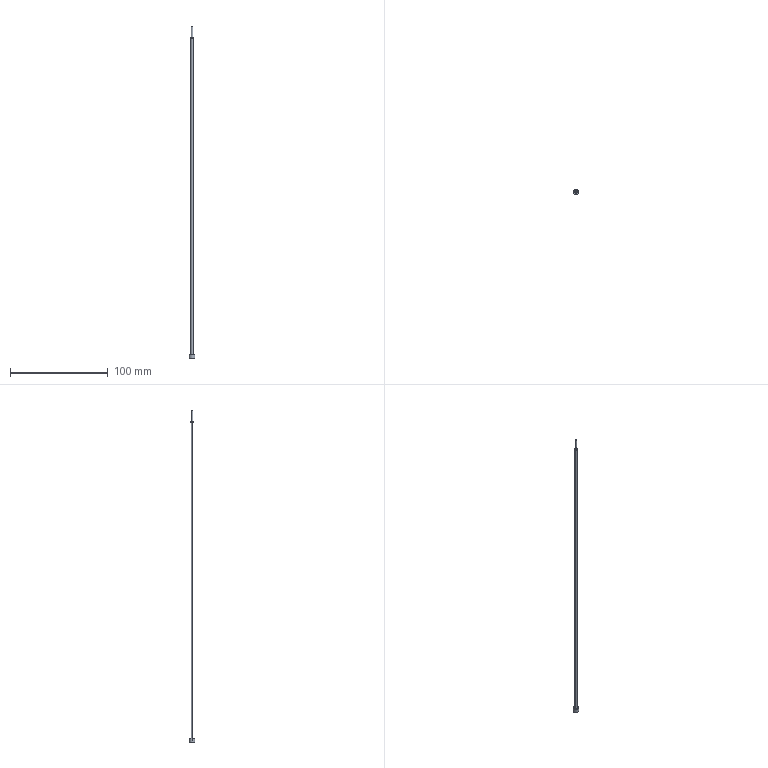Part | Creo | 1 solid | 13 faces | box 6 x 6 x 339.574 mm | volume 2143 mm3 | plane 5 | cone 4 | cylinder 4 | commonest cylinder face diameters 2.8 x2 6 x2
STEP:
#1=CARTESIAN_POINT('',(49.138,56.28,-20.728));
#2=VERTEX_POINT('',#1);
#3=CARTESIAN_POINT('',(46.338,56.28,-20.728));
#4=VERTEX_POINT('',#3);
#5=CARTESIAN_POINT('',(47.738,56.28,-20.728));
#6=DIRECTION('',(0.,0.,1.));
#7=DIRECTION('',(1.,0.,0.));
#8=AXIS2_PLACEMENT_3D('',#5,#6,#7);
#9=CIRCLE('',#8,1.4);
#10=EDGE_CURVE('',#2,#4,#9,.T.);
#11=ORIENTED_EDGE('',*,*,#10,.F.);
#12=CARTESIAN_POINT('',(47.738,56.28,-20.728));
#13=DIRECTION('',(0.,0.,1.));
#14=DIRECTION('',(-1.,0.,0.));
#15=AXIS2_PLACEMENT_3D('',#12,#13,#14);
#16=CIRCLE('',#15,1.4);
#17=EDGE_CURVE('',#4,#2,#16,.T.);
#18=ORIENTED_EDGE('',*,*,#17,.F.);
#19=EDGE_LOOP('',(#11,#18));
#20=FACE_OUTER_BOUND('',#19,.F.);
#21=CARTESIAN_POINT('',(49.1,56.28,-20.728));
#22=VERTEX_POINT('',#21);
#23=CARTESIAN_POINT('',(46.375,56.28,-20.728));
#24=VERTEX_POINT('',#23);
#25=CARTESIAN_POINT('',(47.737,56.28,-20.728));
#26=DIRECTION('',(0.,0.,-1.));
#27=DIRECTION('',(1.,0.,0.));
#28=AXIS2_PLACEMENT_3D('',#25,#26,#27);
#29=CIRCLE('',#28,1.362);
#30=EDGE_CURVE('',#22,#24,#29,.T.);
#31=ORIENTED_EDGE('',*,*,#30,.F.);
#32=CARTESIAN_POINT('',(47.737,56.28,-20.728));
#33=DIRECTION('',(0.,0.,-1.));
#34=DIRECTION('',(-1.,0.,0.));
#35=AXIS2_PLACEMENT_3D('',#32,#33,#34);
#36=CIRCLE('',#35,1.362);
#37=EDGE_CURVE('',#24,#22,#36,.T.);
#38=ORIENTED_EDGE('',*,*,#37,.F.);
#39=EDGE_LOOP('',(#31,#38));
#40=FACE_BOUND('',#39,.F.);
#41=CARTESIAN_POINT('',(47.737,56.318,-20.728));
#42=DIRECTION('',(0.,0.,1.));
#43=DIRECTION('',(1.,0.,0.));
#44=AXIS2_PLACEMENT_3D('',#41,#42,#43);
#45=PLANE('',#44);
#46=ADVANCED_FACE('',(#20,#40),#45,.T.);
#47=CARTESIAN_POINT('',(46.389,56.28,-19.924));
#48=VERTEX_POINT('',#47);
#49=CARTESIAN_POINT('',(49.086,56.28,-19.924));
#50=VERTEX_POINT('',#49);
#51=CARTESIAN_POINT('',(47.737,56.28,-19.924));
#52=DIRECTION('',(0.,0.,1.));
#53=DIRECTION('',(-1.,0.,0.));
#54=AXIS2_PLACEMENT_3D('',#51,#52,#53);
#55=CIRCLE('',#54,1.348);
#56=EDGE_CURVE('',#48,#50,#55,.T.);
#57=ORIENTED_EDGE('',*,*,#56,.T.);
#58=CARTESIAN_POINT('',(49.086,56.28,-19.924));
#59=DIRECTION('',(0.01745,0.,-0.9998));
#60=VECTOR('',#59,0.8041);
#61=LINE('',#58,#60);
#62=EDGE_CURVE('',#50,#22,#61,.T.);
#63=ORIENTED_EDGE('',*,*,#62,.T.);
#64=ORIENTED_EDGE('',*,*,#30,.T.);
#65=CARTESIAN_POINT('',(46.389,56.28,-19.924));
#66=DIRECTION('',(-0.01745,0.,-0.9998));
#67=VECTOR('',#66,0.8041);
#68=LINE('',#65,#67);
#69=EDGE_CURVE('',#48,#24,#68,.T.);
#70=ORIENTED_EDGE('',*,*,#69,.F.);
#71=EDGE_LOOP('',(#57,#63,#64,#70));
#72=FACE_OUTER_BOUND('',#71,.F.);
#73=CARTESIAN_POINT('',(47.737,56.28,-20.326));
#74=DIRECTION('',(0.,0.,-1.));
#75=DIRECTION('',(1.,0.,0.));
#76=AXIS2_PLACEMENT_3D('',#73,#74,#75);
#77=CONICAL_SURFACE('',#76,1.355,1.);
#78=ADVANCED_FACE('',(#72),#77,.T.);
#79=ORIENTED_EDGE('',*,*,#56,.F.);
#80=CARTESIAN_POINT('',(47.737,56.28,-19.924));
#81=DIRECTION('',(0.,0.,1.));
#82=DIRECTION('',(1.,0.,0.));
#83=AXIS2_PLACEMENT_3D('',#80,#81,#82);
#84=CIRCLE('',#83,1.348);
#85=EDGE_CURVE('',#50,#48,#84,.T.);
#86=ORIENTED_EDGE('',*,*,#85,.F.);
#87=EDGE_LOOP('',(#79,#86));
#88=FACE_OUTER_BOUND('',#87,.F.);
#89=CARTESIAN_POINT('',(46.706,56.28,-19.924));
#90=VERTEX_POINT('',#89);
#91=CARTESIAN_POINT('',(48.769,56.28,-19.924));
#92=VERTEX_POINT('',#91);
#93=CARTESIAN_POINT('',(47.737,56.28,-19.924));
#94=DIRECTION('',(0.,0.,-1.));
#95=DIRECTION('',(-1.,0.,0.));
#96=AXIS2_PLACEMENT_3D('',#93,#94,#95);
#97=CIRCLE('',#96,1.031);
#98=EDGE_CURVE('',#90,#92,#97,.T.);
#99=ORIENTED_EDGE('',*,*,#98,.F.);
#100=CARTESIAN_POINT('',(47.737,56.28,-19.924));
#101=DIRECTION('',(0.,0.,-1.));
#102=DIRECTION('',(1.,0.,0.));
#103=AXIS2_PLACEMENT_3D('',#100,#101,#102);
#104=CIRCLE('',#103,1.031);
#105=EDGE_CURVE('',#92,#90,#104,.T.);
#106=ORIENTED_EDGE('',*,*,#105,.F.);
#107=EDGE_LOOP('',(#99,#106));
#108=FACE_BOUND('',#107,.F.);
#109=CARTESIAN_POINT('',(47.737,56.28,-19.924));
#110=DIRECTION('',(0.,0.,-1.));
#111=DIRECTION('',(-1.,0.,0.));
#112=AXIS2_PLACEMENT_3D('',#109,#110,#111);
#113=PLANE('',#112);
#114=ADVANCED_FACE('',(#88,#108),#113,.F.);
#115=CARTESIAN_POINT('',(48.668,56.28,-8.458));
#116=VERTEX_POINT('',#115);
#117=CARTESIAN_POINT('',(46.807,56.28,-8.426));
#118=VERTEX_POINT('',#117);
#119=CARTESIAN_POINT('',(48.668,56.28,-8.458));
#120=CARTESIAN_POINT('',(48.668,56.499,-8.458));
#121=CARTESIAN_POINT('',(48.467,57.021,-8.455));
#122=CARTESIAN_POINT('',(47.738,57.306,-8.442));
#123=CARTESIAN_POINT('',(47.008,57.021,-8.429));
#124=CARTESIAN_POINT('',(46.807,56.499,-8.426));
#125=CARTESIAN_POINT('',(46.807,56.28,-8.426));
#126=B_SPLINE_CURVE_WITH_KNOTS('',3,(#119,#120,#121,#122,#123,#124,#125),.UNSPECIFIED.,.F.,.F.,(4,1,1,1,4),(0.,0.25,0.5,0.75,1.),.UNSPECIFIED.);
#127=EDGE_CURVE('',#116,#118,#126,.T.);
#128=ORIENTED_EDGE('',*,*,#127,.T.);
#129=CARTESIAN_POINT('',(46.807,56.28,-8.426));
#130=DIRECTION('',(-0.008727,0.,-1.));
#131=VECTOR('',#130,11.499);
#132=LINE('',#129,#131);
#133=EDGE_CURVE('',#118,#90,#132,.T.);
#134=ORIENTED_EDGE('',*,*,#133,.T.);
#135=ORIENTED_EDGE('',*,*,#98,.T.);
#136=CARTESIAN_POINT('',(48.668,56.28,-8.458));
#137=DIRECTION('',(0.008727,0.,-1.));
#138=VECTOR('',#137,11.466);
#139=LINE('',#136,#138);
#140=EDGE_CURVE('',#116,#92,#139,.T.);
#141=ORIENTED_EDGE('',*,*,#140,.F.);
#142=EDGE_LOOP('',(#128,#134,#135,#141));
#143=FACE_OUTER_BOUND('',#142,.F.);
#144=CARTESIAN_POINT('',(47.737,56.28,-14.175));
#145=DIRECTION('',(0.,0.,-1.));
#146=DIRECTION('',(-1.,0.,0.));
#147=AXIS2_PLACEMENT_3D('',#144,#145,#146);
#148=CONICAL_SURFACE('',#147,0.9808,0.5);
#149=ADVANCED_FACE('',(#143),#148,.T.);
#150=ORIENTED_EDGE('',*,*,#127,.F.);
#151=CARTESIAN_POINT('',(46.807,56.28,-8.426));
#152=CARTESIAN_POINT('',(46.807,56.061,-8.426));
#153=CARTESIAN_POINT('',(47.008,55.539,-8.429));
#154=CARTESIAN_POINT('',(47.738,55.254,-8.442));
#155=CARTESIAN_POINT('',(48.467,55.539,-8.455));
#156=CARTESIAN_POINT('',(48.668,56.061,-8.458));
#157=CARTESIAN_POINT('',(48.668,56.28,-8.458));
#158=B_SPLINE_CURVE_WITH_KNOTS('',3,(#151,#152,#153,#154,#155,#156,#157),.UNSPECIFIED.,.F.,.F.,(4,1,1,1,4),(0.,0.25,0.5,0.75,1.),.UNSPECIFIED.);
#159=EDGE_CURVE('',#118,#116,#158,.T.);
#160=ORIENTED_EDGE('',*,*,#159,.F.);
#161=EDGE_LOOP('',(#150,#160));
#162=FACE_OUTER_BOUND('',#161,.F.);
#163=CARTESIAN_POINT('',(60.807,51.758,-8.67));
#164=DIRECTION('',(-0.01745,0.,-0.9998));
#165=DIRECTION('',(-0.9998,0.,0.01745));
#166=AXIS2_PLACEMENT_3D('',#163,#164,#165);
#167=PLANE('',#166);
#168=ADVANCED_FACE('',(#162),#167,.F.);
#169=ORIENTED_EDGE('',*,*,#159,.T.);
#170=ORIENTED_EDGE('',*,*,#140,.T.);
#171=ORIENTED_EDGE('',*,*,#105,.T.);
#172=ORIENTED_EDGE('',*,*,#133,.F.);
#173=EDGE_LOOP('',(#169,#170,#171,#172));
#174=FACE_OUTER_BOUND('',#173,.F.);
#175=CARTESIAN_POINT('',(47.737,56.28,-14.175));
#176=DIRECTION('',(0.,0.,-1.));
#177=DIRECTION('',(-1.,0.,0.));
#178=AXIS2_PLACEMENT_3D('',#175,#176,#177);
#179=CONICAL_SURFACE('',#178,0.9808,0.5);
#180=ADVANCED_FACE('',(#174),#179,.T.);
#181=ORIENTED_EDGE('',*,*,#85,.T.);
#182=ORIENTED_EDGE('',*,*,#69,.T.);
#183=ORIENTED_EDGE('',*,*,#37,.T.);
#184=ORIENTED_EDGE('',*,*,#62,.F.);
#185=EDGE_LOOP('',(#181,#182,#183,#184));
#186=FACE_OUTER_BOUND('',#185,.F.);
#187=CARTESIAN_POINT('',(47.737,56.28,-20.326));
#188=DIRECTION('',(0.,0.,-1.));
#189=DIRECTION('',(1.,0.,0.));
#190=AXIS2_PLACEMENT_3D('',#187,#188,#189);
#191=CONICAL_SURFACE('',#190,1.355,1.);
#192=ADVANCED_FACE('',(#186),#191,.T.);
#193=CARTESIAN_POINT('',(46.338,56.28,-344.));
#194=VERTEX_POINT('',#193);
#195=CARTESIAN_POINT('',(49.138,56.28,-344.));
#196=VERTEX_POINT('',#195);
#197=CARTESIAN_POINT('',(47.738,56.28,-344.));
#198=DIRECTION('',(0.,0.,-1.));
#199=DIRECTION('',(-1.,0.,0.));
#200=AXIS2_PLACEMENT_3D('',#197,#198,#199);
#201=CIRCLE('',#200,1.4);
#202=EDGE_CURVE('',#194,#196,#201,.T.);
#203=ORIENTED_EDGE('',*,*,#202,.T.);
#204=CARTESIAN_POINT('',(49.138,56.28,-344.));
#205=DIRECTION('',(0.,0.,1.));
#206=VECTOR('',#205,323.272);
#207=LINE('',#204,#206);
#208=EDGE_CURVE('',#196,#2,#207,.T.);
#209=ORIENTED_EDGE('',*,*,#208,.T.);
#210=ORIENTED_EDGE('',*,*,#10,.T.);
#211=CARTESIAN_POINT('',(46.338,56.28,-344.));
#212=DIRECTION('',(0.,0.,1.));
#213=VECTOR('',#212,323.272);
#214=LINE('',#211,#213);
#215=EDGE_CURVE('',#194,#4,#214,.T.);
#216=ORIENTED_EDGE('',*,*,#215,.F.);
#217=EDGE_LOOP('',(#203,#209,#210,#216));
#218=FACE_OUTER_BOUND('',#217,.F.);
#219=CARTESIAN_POINT('',(47.738,56.28,-428.));
#220=DIRECTION('',(0.,0.,1.));
#221=DIRECTION('',(1.,0.,0.));
#222=AXIS2_PLACEMENT_3D('',#219,#220,#221);
#223=CYLINDRICAL_SURFACE('',#222,1.4);
#224=ADVANCED_FACE('',(#218),#223,.T.);
#225=CARTESIAN_POINT('',(50.738,56.28,-344.));
#226=VERTEX_POINT('',#225);
#227=CARTESIAN_POINT('',(44.738,56.28,-344.));
#228=VERTEX_POINT('',#227);
#229=CARTESIAN_POINT('',(47.738,56.28,-344.));
#230=DIRECTION('',(0.,0.,1.));
#231=DIRECTION('',(1.,0.,0.));
#232=AXIS2_PLACEMENT_3D('',#229,#230,#231);
#233=CIRCLE('',#232,3.);
#234=EDGE_CURVE('',#226,#228,#233,.T.);
#235=ORIENTED_EDGE('',*,*,#234,.F.);
#236=CARTESIAN_POINT('',(47.738,56.28,-344.));
#237=DIRECTION('',(0.,0.,1.));
#238=DIRECTION('',(-1.,0.,0.));
#239=AXIS2_PLACEMENT_3D('',#236,#237,#238);
#240=CIRCLE('',#239,3.);
#241=EDGE_CURVE('',#228,#226,#240,.T.);
#242=ORIENTED_EDGE('',*,*,#241,.F.);
#243=EDGE_LOOP('',(#235,#242));
#244=FACE_OUTER_BOUND('',#243,.F.);
#245=CARTESIAN_POINT('',(47.738,56.28,-344.));
#246=DIRECTION('',(0.,0.,-1.));
#247=DIRECTION('',(1.,0.,0.));
#248=AXIS2_PLACEMENT_3D('',#245,#246,#247);
#249=CIRCLE('',#248,1.4);
#250=EDGE_CURVE('',#196,#194,#249,.T.);
#251=ORIENTED_EDGE('',*,*,#250,.F.);
#252=ORIENTED_EDGE('',*,*,#202,.F.);
#253=EDGE_LOOP('',(#251,#252));
#254=FACE_BOUND('',#253,.F.);
#255=CARTESIAN_POINT('',(47.738,56.28,-344.));
#256=DIRECTION('',(0.,0.,1.));
#257=DIRECTION('',(1.,0.,0.));
#258=AXIS2_PLACEMENT_3D('',#255,#256,#257);
#259=PLANE('',#258);
#260=ADVANCED_FACE('',(#244,#254),#259,.T.);
#261=ORIENTED_EDGE('',*,*,#250,.T.);
#262=ORIENTED_EDGE('',*,*,#215,.T.);
#263=ORIENTED_EDGE('',*,*,#17,.T.);
#264=ORIENTED_EDGE('',*,*,#208,.F.);
#265=EDGE_LOOP('',(#261,#262,#263,#264));
#266=FACE_OUTER_BOUND('',#265,.F.);
#267=CARTESIAN_POINT('',(47.738,56.28,-428.));
#268=DIRECTION('',(0.,0.,1.));
#269=DIRECTION('',(1.,0.,0.));
#270=AXIS2_PLACEMENT_3D('',#267,#268,#269);
#271=CYLINDRICAL_SURFACE('',#270,1.4);
#272=ADVANCED_FACE('',(#266),#271,.T.);
#273=ORIENTED_EDGE('',*,*,#234,.T.);
#274=CARTESIAN_POINT('',(44.738,56.28,-348.));
#275=VERTEX_POINT('',#274);
#276=CARTESIAN_POINT('',(44.738,56.28,-348.));
#277=DIRECTION('',(0.,0.,1.));
#278=VECTOR('',#277,4.);
#279=LINE('',#276,#278);
#280=EDGE_CURVE('',#275,#228,#279,.T.);
#281=ORIENTED_EDGE('',*,*,#280,.F.);
#282=CARTESIAN_POINT('',(50.738,56.28,-348.));
#283=VERTEX_POINT('',#282);
#284=CARTESIAN_POINT('',(47.738,56.28,-348.));
#285=DIRECTION('',(0.,0.,-1.));
#286=DIRECTION('',(-1.,0.,0.));
#287=AXIS2_PLACEMENT_3D('',#284,#285,#286);
#288=CIRCLE('',#287,3.);
#289=EDGE_CURVE('',#275,#283,#288,.T.);
#290=ORIENTED_EDGE('',*,*,#289,.T.);
#291=CARTESIAN_POINT('',(50.738,56.28,-348.));
#292=DIRECTION('',(0.,0.,1.));
#293=VECTOR('',#292,4.);
#294=LINE('',#291,#293);
#295=EDGE_CURVE('',#283,#226,#294,.T.);
#296=ORIENTED_EDGE('',*,*,#295,.T.);
#297=EDGE_LOOP('',(#273,#281,#290,#296));
#298=FACE_OUTER_BOUND('',#297,.F.);
#299=CARTESIAN_POINT('',(47.738,56.28,-348.));
#300=DIRECTION('',(0.,0.,1.));
#301=DIRECTION('',(1.,0.,0.));
#302=AXIS2_PLACEMENT_3D('',#299,#300,#301);
#303=CYLINDRICAL_SURFACE('',#302,3.);
#304=ADVANCED_FACE('',(#298),#303,.T.);
#305=ORIENTED_EDGE('',*,*,#241,.T.);
#306=ORIENTED_EDGE('',*,*,#295,.F.);
#307=CARTESIAN_POINT('',(47.738,56.28,-348.));
#308=DIRECTION('',(0.,0.,-1.));
#309=DIRECTION('',(1.,0.,0.));
#310=AXIS2_PLACEMENT_3D('',#307,#308,#309);
#311=CIRCLE('',#310,3.);
#312=EDGE_CURVE('',#283,#275,#311,.T.);
#313=ORIENTED_EDGE('',*,*,#312,.T.);
#314=ORIENTED_EDGE('',*,*,#280,.T.);
#315=EDGE_LOOP('',(#305,#306,#313,#314));
#316=FACE_OUTER_BOUND('',#315,.F.);
#317=CARTESIAN_POINT('',(47.738,56.28,-348.));
#318=DIRECTION('',(0.,0.,1.));
#319=DIRECTION('',(1.,0.,0.));
#320=AXIS2_PLACEMENT_3D('',#317,#318,#319);
#321=CYLINDRICAL_SURFACE('',#320,3.);
#322=ADVANCED_FACE('',(#316),#321,.T.);
#323=ORIENTED_EDGE('',*,*,#312,.F.);
#324=ORIENTED_EDGE('',*,*,#289,.F.);
#325=EDGE_LOOP('',(#323,#324));
#326=FACE_OUTER_BOUND('',#325,.F.);
#327=CARTESIAN_POINT('',(58.,64.995,-348.));
#328=DIRECTION('',(0.,0.,1.));
#329=DIRECTION('',(-1.,0.,0.));
#330=AXIS2_PLACEMENT_3D('',#327,#328,#329);
#331=PLANE('',#330);
#332=ADVANCED_FACE('',(#326),#331,.F.);
#333=CLOSED_SHELL('',(#46,#78,#114,#149,#168,#180,#192,#224,#260,#272,#304,#322,#332));
#334=MANIFOLD_SOLID_BREP('',#333);
#335=(LENGTH_UNIT()NAMED_UNIT(*)SI_UNIT(.MILLI.,.METRE.));
#336=UNCERTAINTY_MEASURE_WITH_UNIT(LENGTH_MEASURE(0.03397),#335,'','');
#337=(NAMED_UNIT(*)PLANE_ANGLE_UNIT()SI_UNIT($,.RADIAN.));
#338=PLANE_ANGLE_MEASURE_WITH_UNIT(PLANE_ANGLE_MEASURE(0.01745),#337);
#339=(CONVERSION_BASED_UNIT('DEGREE',#338)NAMED_UNIT(*)PLANE_ANGLE_UNIT());
#340=(NAMED_UNIT(*)SI_UNIT($,.STERADIAN.)SOLID_ANGLE_UNIT());
#341=(GEOMETRIC_REPRESENTATION_CONTEXT(3)GLOBAL_UNCERTAINTY_ASSIGNED_CONTEXT((#336))GLOBAL_UNIT_ASSIGNED_CONTEXT((#335,#339,#340))REPRESENTATION_CONTEXT('',''));
#342=ADVANCED_BREP_SHAPE_REPRESENTATION('',(#334),#341);